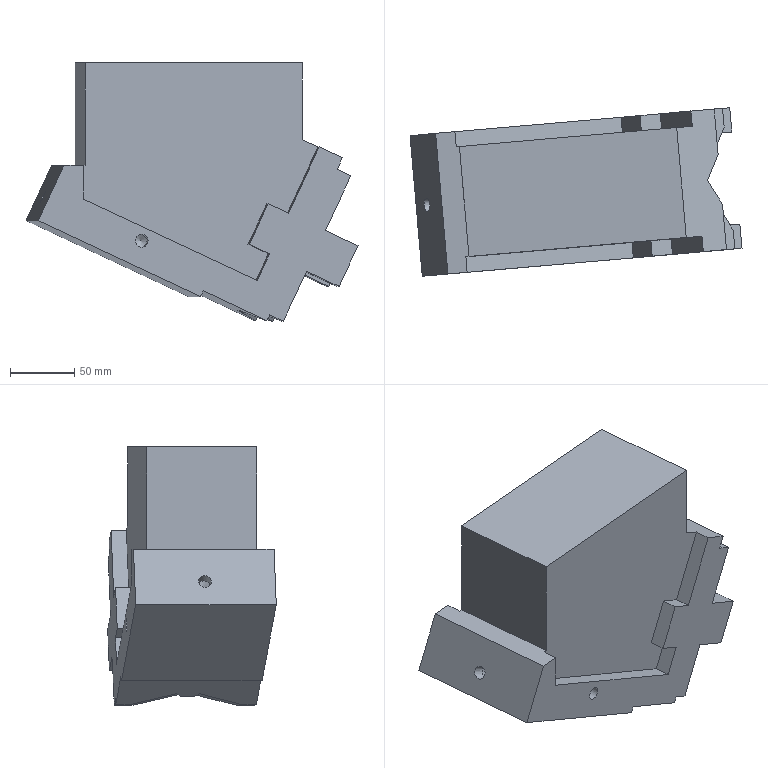Part | NX | features MAIN_BODY 2 | 1 solid | 71 faces | box 258.808 x 131.385 x 201.374 mm | volume 3021281 mm3 | plane 57 | cylinder 9 | cone 5 | commonest cylinder face diameters 10 x3 6.8 x2 8 x2 15 x2